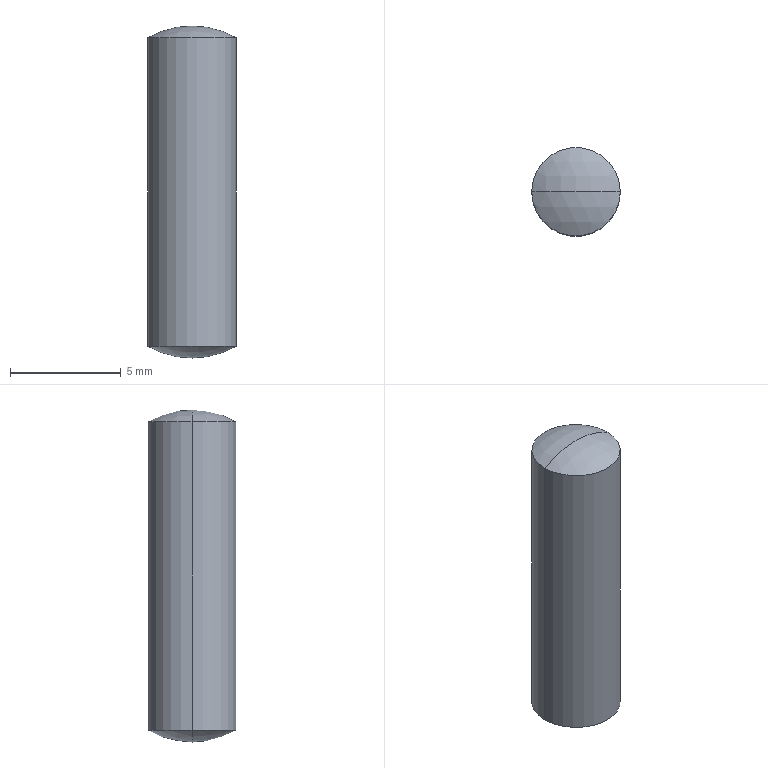Part | SolidWorks | features Attribute 1, Revolution 1 | 1 solid | 6 faces | box 4 x 4 x 15 mm | volume 181.922 mm3 | sphere 4 | cylinder 2 | commonest cylinder face diameters 4 x2
STEP:
#1=CARTESIAN_POINT('',(-2.,0.,6.464));
#2=VERTEX_POINT('',#1);
#3=CARTESIAN_POINT('',(2.,0.,6.464));
#4=VERTEX_POINT('',#3);
#5=CARTESIAN_POINT('',(0.,0.,6.464));
#6=DIRECTION('',(0.,0.,-1.));
#7=DIRECTION('',(-1.,0.,0.));
#8=AXIS2_PLACEMENT_3D('',#5,#6,#7);
#9=CIRCLE('',#8,2.);
#10=EDGE_CURVE('',#2,#4,#9,.T.);
#11=ORIENTED_EDGE('',*,*,#10,.T.);
#12=CARTESIAN_POINT('',(2.,0.,-7.464));
#13=VERTEX_POINT('',#12);
#14=CARTESIAN_POINT('',(2.,0.,-47.537));
#15=DIRECTION('',(0.,0.,-1.));
#16=VECTOR('',#15,1000.);
#17=LINE('',#14,#16);
#18=EDGE_CURVE('',#4,#13,#17,.T.);
#19=ORIENTED_EDGE('',*,*,#18,.T.);
#20=CARTESIAN_POINT('',(-2.,0.,-7.464));
#21=VERTEX_POINT('',#20);
#22=CARTESIAN_POINT('',(0.,0.,-7.464));
#23=DIRECTION('',(0.,0.,-1.));
#24=DIRECTION('',(-1.,0.,0.));
#25=AXIS2_PLACEMENT_3D('',#22,#23,#24);
#26=CIRCLE('',#25,2.);
#27=EDGE_CURVE('',#21,#13,#26,.T.);
#28=ORIENTED_EDGE('',*,*,#27,.F.);
#29=CARTESIAN_POINT('',(-2.,0.,-47.537));
#30=DIRECTION('',(0.,0.,-1.));
#31=VECTOR('',#30,1000.);
#32=LINE('',#29,#31);
#33=EDGE_CURVE('',#2,#21,#32,.T.);
#34=ORIENTED_EDGE('',*,*,#33,.F.);
#35=EDGE_LOOP('',(#11,#19,#28,#34));
#36=FACE_OUTER_BOUND('',#35,.T.);
#37=CARTESIAN_POINT('',(0.,0.,-47.537));
#38=DIRECTION('',(0.,0.,-1.));
#39=DIRECTION('',(-1.,0.,0.));
#40=AXIS2_PLACEMENT_3D('',#37,#38,#39);
#41=CYLINDRICAL_SURFACE('',#40,2.);
#42=ADVANCED_FACE('',(#36),#41,.T.);
#43=CARTESIAN_POINT('',(0.,0.,7.));
#44=VERTEX_POINT('',#43);
#45=CARTESIAN_POINT('',(0.,0.,3.));
#46=DIRECTION('',(0.,1.,0.));
#47=DIRECTION('',(0.,0.,1.));
#48=AXIS2_PLACEMENT_3D('',#45,#46,#47);
#49=CIRCLE('',#48,4.);
#50=EDGE_CURVE('',#44,#4,#49,.T.);
#51=ORIENTED_EDGE('',*,*,#50,.F.);
#52=CARTESIAN_POINT('',(0.,0.,3.));
#53=DIRECTION('',(0.,-1.,0.));
#54=DIRECTION('',(1.,0.,0.));
#55=AXIS2_PLACEMENT_3D('',#52,#53,#54);
#56=CIRCLE('',#55,4.);
#57=EDGE_CURVE('',#44,#2,#56,.T.);
#58=ORIENTED_EDGE('',*,*,#57,.T.);
#59=CARTESIAN_POINT('',(0.,0.,6.464));
#60=DIRECTION('',(0.,0.,-1.));
#61=DIRECTION('',(-1.,0.,0.));
#62=AXIS2_PLACEMENT_3D('',#59,#60,#61);
#63=CIRCLE('',#62,2.);
#64=EDGE_CURVE('',#4,#2,#63,.T.);
#65=ORIENTED_EDGE('',*,*,#64,.F.);
#66=EDGE_LOOP('',(#51,#58,#65));
#67=FACE_OUTER_BOUND('',#66,.T.);
#68=CARTESIAN_POINT('',(0.,0.,3.));
#69=DIRECTION('',(0.,-1.,0.));
#70=DIRECTION('',(1.,0.,0.));
#71=AXIS2_PLACEMENT_3D('',#68,#69,#70);
#72=SPHERICAL_SURFACE('',#71,4.);
#73=ADVANCED_FACE('',(#67),#72,.T.);
#74=ORIENTED_EDGE('',*,*,#27,.T.);
#75=CARTESIAN_POINT('',(0.,0.,-8.));
#76=VERTEX_POINT('',#75);
#77=CARTESIAN_POINT('',(0.,0.,-4.));
#78=DIRECTION('',(0.,1.,0.));
#79=DIRECTION('',(-1.,0.,0.));
#80=AXIS2_PLACEMENT_3D('',#77,#78,#79);
#81=CIRCLE('',#80,4.);
#82=EDGE_CURVE('',#13,#76,#81,.T.);
#83=ORIENTED_EDGE('',*,*,#82,.T.);
#84=CARTESIAN_POINT('',(0.,0.,-4.));
#85=DIRECTION('',(0.,-1.,0.));
#86=DIRECTION('',(0.,0.,-1.));
#87=AXIS2_PLACEMENT_3D('',#84,#85,#86);
#88=CIRCLE('',#87,4.);
#89=EDGE_CURVE('',#21,#76,#88,.T.);
#90=ORIENTED_EDGE('',*,*,#89,.F.);
#91=EDGE_LOOP('',(#74,#83,#90));
#92=FACE_OUTER_BOUND('',#91,.T.);
#93=CARTESIAN_POINT('',(0.,0.,-4.));
#94=DIRECTION('',(0.,1.,0.));
#95=DIRECTION('',(-1.,0.,0.));
#96=AXIS2_PLACEMENT_3D('',#93,#94,#95);
#97=SPHERICAL_SURFACE('',#96,4.);
#98=ADVANCED_FACE('',(#92),#97,.T.);
#99=ORIENTED_EDGE('',*,*,#82,.F.);
#100=CARTESIAN_POINT('',(0.,0.,-7.464));
#101=DIRECTION('',(0.,0.,-1.));
#102=DIRECTION('',(-1.,0.,0.));
#103=AXIS2_PLACEMENT_3D('',#100,#101,#102);
#104=CIRCLE('',#103,2.);
#105=EDGE_CURVE('',#13,#21,#104,.T.);
#106=ORIENTED_EDGE('',*,*,#105,.T.);
#107=ORIENTED_EDGE('',*,*,#89,.T.);
#108=EDGE_LOOP('',(#99,#106,#107));
#109=FACE_OUTER_BOUND('',#108,.T.);
#110=CARTESIAN_POINT('',(0.,0.,-4.));
#111=DIRECTION('',(0.,1.,0.));
#112=DIRECTION('',(-1.,0.,0.));
#113=AXIS2_PLACEMENT_3D('',#110,#111,#112);
#114=SPHERICAL_SURFACE('',#113,4.);
#115=ADVANCED_FACE('',(#109),#114,.T.);
#116=ORIENTED_EDGE('',*,*,#57,.F.);
#117=ORIENTED_EDGE('',*,*,#50,.T.);
#118=ORIENTED_EDGE('',*,*,#10,.F.);
#119=EDGE_LOOP('',(#116,#117,#118));
#120=FACE_OUTER_BOUND('',#119,.T.);
#121=CARTESIAN_POINT('',(0.,0.,3.));
#122=DIRECTION('',(0.,-1.,0.));
#123=DIRECTION('',(1.,0.,0.));
#124=AXIS2_PLACEMENT_3D('',#121,#122,#123);
#125=SPHERICAL_SURFACE('',#124,4.);
#126=ADVANCED_FACE('',(#120),#125,.T.);
#127=ORIENTED_EDGE('',*,*,#18,.F.);
#128=ORIENTED_EDGE('',*,*,#64,.T.);
#129=ORIENTED_EDGE('',*,*,#33,.T.);
#130=ORIENTED_EDGE('',*,*,#105,.F.);
#131=EDGE_LOOP('',(#127,#128,#129,#130));
#132=FACE_OUTER_BOUND('',#131,.T.);
#133=CARTESIAN_POINT('',(0.,0.,-47.537));
#134=DIRECTION('',(0.,0.,-1.));
#135=DIRECTION('',(-1.,0.,0.));
#136=AXIS2_PLACEMENT_3D('',#133,#134,#135);
#137=CYLINDRICAL_SURFACE('',#136,2.);
#138=ADVANCED_FACE('',(#132),#137,.T.);
#139=CLOSED_SHELL('',(#42,#73,#98,#115,#126,#138));
#140=MANIFOLD_SOLID_BREP('',#139);
#141=CARTESIAN_POINT('',(0.,0.,0.));
#142=DIRECTION('',(0.,0.,1.));
#143=DIRECTION('',(1.,0.,0.));
#144=AXIS2_PLACEMENT_3D('',#141,#142,#143);
#145=(LENGTH_UNIT()NAMED_UNIT(*)SI_UNIT(.MILLI.,.METRE.));
#146=UNCERTAINTY_MEASURE_WITH_UNIT(LENGTH_MEASURE(0.00001),#145,'','');
#147=(NAMED_UNIT(*)PLANE_ANGLE_UNIT()SI_UNIT($,.RADIAN.));
#148=(NAMED_UNIT(*)SI_UNIT($,.STERADIAN.)SOLID_ANGLE_UNIT());
#149=(GEOMETRIC_REPRESENTATION_CONTEXT(3)GLOBAL_UNCERTAINTY_ASSIGNED_CONTEXT((#146))GLOBAL_UNIT_ASSIGNED_CONTEXT((#145,#147,#148))REPRESENTATION_CONTEXT('',''));
#150=ADVANCED_BREP_SHAPE_REPRESENTATION('',(#140,#144),#149);